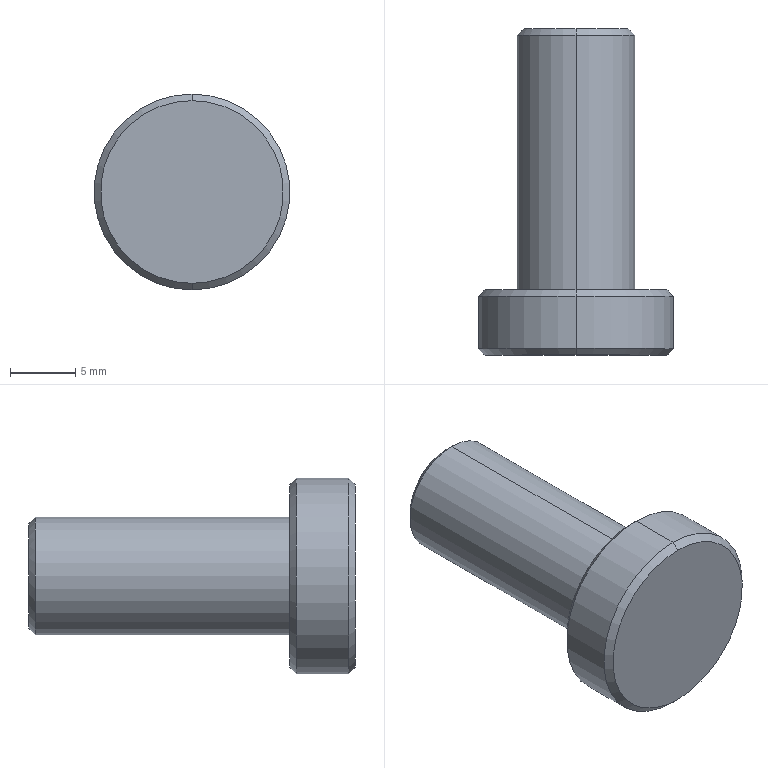Part | SolidWorks | features Chamfer 1, Revolution 1 | 1 solid | 13 faces | box 15 x 25 x 15 mm | volume 2141 mm3 | cone 6 | cylinder 4 | plane 3 | commonest cylinder face diameters 9 x2 15 x2
STEP:
#1=CARTESIAN_POINT('',(0.,25.,4.));
#2=VERTEX_POINT('',#1);
#3=CARTESIAN_POINT('',(0.,25.,-4.));
#4=VERTEX_POINT('',#3);
#5=CARTESIAN_POINT('',(0.,25.,0.));
#6=DIRECTION('',(0.,1.,0.));
#7=DIRECTION('',(0.,0.,1.));
#8=AXIS2_PLACEMENT_3D('',#5,#6,#7);
#9=CIRCLE('',#8,4.);
#10=EDGE_CURVE('',#2,#4,#9,.T.);
#11=ORIENTED_EDGE('',*,*,#10,.F.);
#12=CARTESIAN_POINT('',(0.,24.5,4.5));
#13=VERTEX_POINT('',#12);
#14=CARTESIAN_POINT('',(0.,24.5,4.5));
#15=DIRECTION('',(0.,-0.7071,0.7071));
#16=VECTOR('',#15,1000.);
#17=LINE('',#14,#16);
#18=EDGE_CURVE('',#2,#13,#17,.T.);
#19=ORIENTED_EDGE('',*,*,#18,.T.);
#20=CARTESIAN_POINT('',(0.,24.5,-4.5));
#21=VERTEX_POINT('',#20);
#22=CARTESIAN_POINT('',(0.,24.5,0.));
#23=DIRECTION('',(0.,-1.,0.));
#24=DIRECTION('',(0.,0.,1.));
#25=AXIS2_PLACEMENT_3D('',#22,#23,#24);
#26=CIRCLE('',#25,4.5);
#27=EDGE_CURVE('',#21,#13,#26,.T.);
#28=ORIENTED_EDGE('',*,*,#27,.F.);
#29=CARTESIAN_POINT('',(0.,24.5,-4.5));
#30=DIRECTION('',(0.,-0.7071,-0.7071));
#31=VECTOR('',#30,1000.);
#32=LINE('',#29,#31);
#33=EDGE_CURVE('',#4,#21,#32,.T.);
#34=ORIENTED_EDGE('',*,*,#33,.F.);
#35=EDGE_LOOP('',(#11,#19,#28,#34));
#36=FACE_OUTER_BOUND('',#35,.T.);
#37=CARTESIAN_POINT('',(0.,24.5,0.));
#38=DIRECTION('',(0.,-1.,0.));
#39=DIRECTION('',(0.,0.,-1.));
#40=AXIS2_PLACEMENT_3D('',#37,#38,#39);
#41=CONICAL_SURFACE('',#40,4.5,0.7854);
#42=ADVANCED_FACE('',(#36),#41,.T.);
#43=CARTESIAN_POINT('',(0.,5.,7.));
#44=VERTEX_POINT('',#43);
#45=CARTESIAN_POINT('',(0.,5.,-7.));
#46=VERTEX_POINT('',#45);
#47=CARTESIAN_POINT('',(0.,5.,0.));
#48=DIRECTION('',(0.,1.,0.));
#49=DIRECTION('',(0.,0.,1.));
#50=AXIS2_PLACEMENT_3D('',#47,#48,#49);
#51=CIRCLE('',#50,7.);
#52=EDGE_CURVE('',#44,#46,#51,.T.);
#53=ORIENTED_EDGE('',*,*,#52,.F.);
#54=CARTESIAN_POINT('',(0.,4.5,7.5));
#55=VERTEX_POINT('',#54);
#56=CARTESIAN_POINT('',(0.,4.5,7.5));
#57=DIRECTION('',(0.,-0.7071,0.7071));
#58=VECTOR('',#57,1000.);
#59=LINE('',#56,#58);
#60=EDGE_CURVE('',#44,#55,#59,.T.);
#61=ORIENTED_EDGE('',*,*,#60,.T.);
#62=CARTESIAN_POINT('',(0.,4.5,-7.5));
#63=VERTEX_POINT('',#62);
#64=CARTESIAN_POINT('',(0.,4.5,0.));
#65=DIRECTION('',(0.,-1.,0.));
#66=DIRECTION('',(0.,0.,1.));
#67=AXIS2_PLACEMENT_3D('',#64,#65,#66);
#68=CIRCLE('',#67,7.5);
#69=EDGE_CURVE('',#63,#55,#68,.T.);
#70=ORIENTED_EDGE('',*,*,#69,.F.);
#71=CARTESIAN_POINT('',(0.,4.5,-7.5));
#72=DIRECTION('',(0.,-0.7071,-0.7071));
#73=VECTOR('',#72,1000.);
#74=LINE('',#71,#73);
#75=EDGE_CURVE('',#46,#63,#74,.T.);
#76=ORIENTED_EDGE('',*,*,#75,.F.);
#77=EDGE_LOOP('',(#53,#61,#70,#76));
#78=FACE_OUTER_BOUND('',#77,.T.);
#79=CARTESIAN_POINT('',(0.,4.5,0.));
#80=DIRECTION('',(0.,-1.,0.));
#81=DIRECTION('',(0.,0.,-1.));
#82=AXIS2_PLACEMENT_3D('',#79,#80,#81);
#83=CONICAL_SURFACE('',#82,7.5,0.7854);
#84=ADVANCED_FACE('',(#78),#83,.T.);
#85=CARTESIAN_POINT('',(0.,0.,-7.));
#86=VERTEX_POINT('',#85);
#87=CARTESIAN_POINT('',(0.,0.,7.));
#88=VERTEX_POINT('',#87);
#89=CARTESIAN_POINT('',(0.,0.,0.));
#90=DIRECTION('',(0.,-1.,0.));
#91=DIRECTION('',(0.,0.,-1.));
#92=AXIS2_PLACEMENT_3D('',#89,#90,#91);
#93=CIRCLE('',#92,7.);
#94=EDGE_CURVE('',#86,#88,#93,.T.);
#95=ORIENTED_EDGE('',*,*,#94,.F.);
#96=CARTESIAN_POINT('',(0.,0.5,-7.5));
#97=VERTEX_POINT('',#96);
#98=CARTESIAN_POINT('',(0.,0.,-7.));
#99=DIRECTION('',(0.,0.7071,-0.7071));
#100=VECTOR('',#99,1000.);
#101=LINE('',#98,#100);
#102=EDGE_CURVE('',#86,#97,#101,.T.);
#103=ORIENTED_EDGE('',*,*,#102,.T.);
#104=CARTESIAN_POINT('',(0.,0.5,7.5));
#105=VERTEX_POINT('',#104);
#106=CARTESIAN_POINT('',(0.,0.5,0.));
#107=DIRECTION('',(0.,1.,0.));
#108=DIRECTION('',(0.,0.,-1.));
#109=AXIS2_PLACEMENT_3D('',#106,#107,#108);
#110=CIRCLE('',#109,7.5);
#111=EDGE_CURVE('',#105,#97,#110,.T.);
#112=ORIENTED_EDGE('',*,*,#111,.F.);
#113=CARTESIAN_POINT('',(0.,0.,7.));
#114=DIRECTION('',(0.,0.7071,0.7071));
#115=VECTOR('',#114,1000.);
#116=LINE('',#113,#115);
#117=EDGE_CURVE('',#88,#105,#116,.T.);
#118=ORIENTED_EDGE('',*,*,#117,.F.);
#119=EDGE_LOOP('',(#95,#103,#112,#118));
#120=FACE_OUTER_BOUND('',#119,.T.);
#121=CARTESIAN_POINT('',(0.,0.,0.));
#122=DIRECTION('',(0.,1.,0.));
#123=DIRECTION('',(0.,0.,1.));
#124=AXIS2_PLACEMENT_3D('',#121,#122,#123);
#125=CONICAL_SURFACE('',#124,7.,0.7854);
#126=ADVANCED_FACE('',(#120),#125,.T.);
#127=ORIENTED_EDGE('',*,*,#69,.T.);
#128=CARTESIAN_POINT('',(0.,0.,7.5));
#129=DIRECTION('',(0.,-1.,0.));
#130=VECTOR('',#129,1000.);
#131=LINE('',#128,#130);
#132=EDGE_CURVE('',#55,#105,#131,.T.);
#133=ORIENTED_EDGE('',*,*,#132,.T.);
#134=ORIENTED_EDGE('',*,*,#111,.T.);
#135=CARTESIAN_POINT('',(0.,0.,-7.5));
#136=DIRECTION('',(0.,-1.,0.));
#137=VECTOR('',#136,1000.);
#138=LINE('',#135,#137);
#139=EDGE_CURVE('',#63,#97,#138,.T.);
#140=ORIENTED_EDGE('',*,*,#139,.F.);
#141=EDGE_LOOP('',(#127,#133,#134,#140));
#142=FACE_OUTER_BOUND('',#141,.T.);
#143=CARTESIAN_POINT('',(0.,0.,0.));
#144=DIRECTION('',(0.,-1.,0.));
#145=DIRECTION('',(0.,0.,-1.));
#146=AXIS2_PLACEMENT_3D('',#143,#144,#145);
#147=CYLINDRICAL_SURFACE('',#146,7.5);
#148=ADVANCED_FACE('',(#142),#147,.T.);
#149=ORIENTED_EDGE('',*,*,#27,.T.);
#150=CARTESIAN_POINT('',(0.,5.,4.5));
#151=VERTEX_POINT('',#150);
#152=CARTESIAN_POINT('',(0.,0.,4.5));
#153=DIRECTION('',(0.,-1.,0.));
#154=VECTOR('',#153,1000.);
#155=LINE('',#152,#154);
#156=EDGE_CURVE('',#13,#151,#155,.T.);
#157=ORIENTED_EDGE('',*,*,#156,.T.);
#158=CARTESIAN_POINT('',(0.,5.,-4.5));
#159=VERTEX_POINT('',#158);
#160=CARTESIAN_POINT('',(0.,5.,0.));
#161=DIRECTION('',(0.,-1.,0.));
#162=DIRECTION('',(0.,0.,-1.));
#163=AXIS2_PLACEMENT_3D('',#160,#161,#162);
#164=CIRCLE('',#163,4.5);
#165=EDGE_CURVE('',#159,#151,#164,.T.);
#166=ORIENTED_EDGE('',*,*,#165,.F.);
#167=CARTESIAN_POINT('',(0.,0.,-4.5));
#168=DIRECTION('',(0.,-1.,0.));
#169=VECTOR('',#168,1000.);
#170=LINE('',#167,#169);
#171=EDGE_CURVE('',#21,#159,#170,.T.);
#172=ORIENTED_EDGE('',*,*,#171,.F.);
#173=EDGE_LOOP('',(#149,#157,#166,#172));
#174=FACE_OUTER_BOUND('',#173,.T.);
#175=CARTESIAN_POINT('',(0.,0.,0.));
#176=DIRECTION('',(0.,-1.,0.));
#177=DIRECTION('',(0.,0.,-1.));
#178=AXIS2_PLACEMENT_3D('',#175,#176,#177);
#179=CYLINDRICAL_SURFACE('',#178,4.5);
#180=ADVANCED_FACE('',(#174),#179,.T.);
#181=CARTESIAN_POINT('',(0.,25.,0.));
#182=DIRECTION('',(0.,1.,0.));
#183=DIRECTION('',(0.,0.,1.));
#184=AXIS2_PLACEMENT_3D('',#181,#182,#183);
#185=CIRCLE('',#184,4.);
#186=EDGE_CURVE('',#4,#2,#185,.T.);
#187=ORIENTED_EDGE('',*,*,#186,.T.);
#188=ORIENTED_EDGE('',*,*,#10,.T.);
#189=EDGE_LOOP('',(#187,#188));
#190=FACE_OUTER_BOUND('',#189,.T.);
#191=CARTESIAN_POINT('',(0.,25.,0.));
#192=DIRECTION('',(0.,1.,0.));
#193=DIRECTION('',(0.,0.,1.));
#194=AXIS2_PLACEMENT_3D('',#191,#192,#193);
#195=PLANE('',#194);
#196=ADVANCED_FACE('',(#190),#195,.T.);
#197=ORIENTED_EDGE('',*,*,#156,.F.);
#198=CARTESIAN_POINT('',(0.,24.5,0.));
#199=DIRECTION('',(0.,-1.,0.));
#200=DIRECTION('',(0.,0.,1.));
#201=AXIS2_PLACEMENT_3D('',#198,#199,#200);
#202=CIRCLE('',#201,4.5);
#203=EDGE_CURVE('',#13,#21,#202,.T.);
#204=ORIENTED_EDGE('',*,*,#203,.T.);
#205=ORIENTED_EDGE('',*,*,#171,.T.);
#206=CARTESIAN_POINT('',(0.,5.,0.));
#207=DIRECTION('',(0.,-1.,0.));
#208=DIRECTION('',(0.,0.,-1.));
#209=AXIS2_PLACEMENT_3D('',#206,#207,#208);
#210=CIRCLE('',#209,4.5);
#211=EDGE_CURVE('',#151,#159,#210,.T.);
#212=ORIENTED_EDGE('',*,*,#211,.F.);
#213=EDGE_LOOP('',(#197,#204,#205,#212));
#214=FACE_OUTER_BOUND('',#213,.T.);
#215=CARTESIAN_POINT('',(0.,0.,0.));
#216=DIRECTION('',(0.,-1.,0.));
#217=DIRECTION('',(0.,0.,-1.));
#218=AXIS2_PLACEMENT_3D('',#215,#216,#217);
#219=CYLINDRICAL_SURFACE('',#218,4.5);
#220=ADVANCED_FACE('',(#214),#219,.T.);
#221=CARTESIAN_POINT('',(0.,5.,0.));
#222=DIRECTION('',(0.,1.,0.));
#223=DIRECTION('',(0.,0.,1.));
#224=AXIS2_PLACEMENT_3D('',#221,#222,#223);
#225=CIRCLE('',#224,7.);
#226=EDGE_CURVE('',#46,#44,#225,.T.);
#227=ORIENTED_EDGE('',*,*,#226,.T.);
#228=ORIENTED_EDGE('',*,*,#52,.T.);
#229=EDGE_LOOP('',(#227,#228));
#230=FACE_OUTER_BOUND('',#229,.T.);
#231=ORIENTED_EDGE('',*,*,#165,.T.);
#232=ORIENTED_EDGE('',*,*,#211,.T.);
#233=EDGE_LOOP('',(#231,#232));
#234=FACE_BOUND('',#233,.T.);
#235=CARTESIAN_POINT('',(0.,5.,-4.5));
#236=DIRECTION('',(0.,1.,0.));
#237=DIRECTION('',(0.,0.,1.));
#238=AXIS2_PLACEMENT_3D('',#235,#236,#237);
#239=PLANE('',#238);
#240=ADVANCED_FACE('',(#230,#234),#239,.T.);
#241=ORIENTED_EDGE('',*,*,#132,.F.);
#242=CARTESIAN_POINT('',(0.,4.5,0.));
#243=DIRECTION('',(0.,-1.,0.));
#244=DIRECTION('',(0.,0.,1.));
#245=AXIS2_PLACEMENT_3D('',#242,#243,#244);
#246=CIRCLE('',#245,7.5);
#247=EDGE_CURVE('',#55,#63,#246,.T.);
#248=ORIENTED_EDGE('',*,*,#247,.T.);
#249=ORIENTED_EDGE('',*,*,#139,.T.);
#250=CARTESIAN_POINT('',(0.,0.5,0.));
#251=DIRECTION('',(0.,1.,0.));
#252=DIRECTION('',(0.,0.,-1.));
#253=AXIS2_PLACEMENT_3D('',#250,#251,#252);
#254=CIRCLE('',#253,7.5);
#255=EDGE_CURVE('',#97,#105,#254,.T.);
#256=ORIENTED_EDGE('',*,*,#255,.T.);
#257=EDGE_LOOP('',(#241,#248,#249,#256));
#258=FACE_OUTER_BOUND('',#257,.T.);
#259=CARTESIAN_POINT('',(0.,0.,0.));
#260=DIRECTION('',(0.,-1.,0.));
#261=DIRECTION('',(0.,0.,-1.));
#262=AXIS2_PLACEMENT_3D('',#259,#260,#261);
#263=CYLINDRICAL_SURFACE('',#262,7.5);
#264=ADVANCED_FACE('',(#258),#263,.T.);
#265=CARTESIAN_POINT('',(0.,0.,0.));
#266=DIRECTION('',(0.,-1.,0.));
#267=DIRECTION('',(0.,0.,-1.));
#268=AXIS2_PLACEMENT_3D('',#265,#266,#267);
#269=CIRCLE('',#268,7.);
#270=EDGE_CURVE('',#88,#86,#269,.T.);
#271=ORIENTED_EDGE('',*,*,#270,.T.);
#272=ORIENTED_EDGE('',*,*,#94,.T.);
#273=EDGE_LOOP('',(#271,#272));
#274=FACE_OUTER_BOUND('',#273,.T.);
#275=CARTESIAN_POINT('',(0.,0.,-7.5));
#276=DIRECTION('',(0.,-1.,0.));
#277=DIRECTION('',(0.,0.,-1.));
#278=AXIS2_PLACEMENT_3D('',#275,#276,#277);
#279=PLANE('',#278);
#280=ADVANCED_FACE('',(#274),#279,.T.);
#281=ORIENTED_EDGE('',*,*,#102,.F.);
#282=ORIENTED_EDGE('',*,*,#270,.F.);
#283=ORIENTED_EDGE('',*,*,#117,.T.);
#284=ORIENTED_EDGE('',*,*,#255,.F.);
#285=EDGE_LOOP('',(#281,#282,#283,#284));
#286=FACE_OUTER_BOUND('',#285,.T.);
#287=CARTESIAN_POINT('',(0.,0.,0.));
#288=DIRECTION('',(0.,1.,0.));
#289=DIRECTION('',(0.,0.,1.));
#290=AXIS2_PLACEMENT_3D('',#287,#288,#289);
#291=CONICAL_SURFACE('',#290,7.,0.7854);
#292=ADVANCED_FACE('',(#286),#291,.T.);
#293=ORIENTED_EDGE('',*,*,#60,.F.);
#294=ORIENTED_EDGE('',*,*,#226,.F.);
#295=ORIENTED_EDGE('',*,*,#75,.T.);
#296=ORIENTED_EDGE('',*,*,#247,.F.);
#297=EDGE_LOOP('',(#293,#294,#295,#296));
#298=FACE_OUTER_BOUND('',#297,.T.);
#299=CARTESIAN_POINT('',(0.,4.5,0.));
#300=DIRECTION('',(0.,-1.,0.));
#301=DIRECTION('',(0.,0.,-1.));
#302=AXIS2_PLACEMENT_3D('',#299,#300,#301);
#303=CONICAL_SURFACE('',#302,7.5,0.7854);
#304=ADVANCED_FACE('',(#298),#303,.T.);
#305=ORIENTED_EDGE('',*,*,#18,.F.);
#306=ORIENTED_EDGE('',*,*,#186,.F.);
#307=ORIENTED_EDGE('',*,*,#33,.T.);
#308=ORIENTED_EDGE('',*,*,#203,.F.);
#309=EDGE_LOOP('',(#305,#306,#307,#308));
#310=FACE_OUTER_BOUND('',#309,.T.);
#311=CARTESIAN_POINT('',(0.,24.5,0.));
#312=DIRECTION('',(0.,-1.,0.));
#313=DIRECTION('',(0.,0.,-1.));
#314=AXIS2_PLACEMENT_3D('',#311,#312,#313);
#315=CONICAL_SURFACE('',#314,4.5,0.7854);
#316=ADVANCED_FACE('',(#310),#315,.T.);
#317=CLOSED_SHELL('',(#42,#84,#126,#148,#180,#196,#220,#240,#264,#280,#292,#304,#316));
#318=MANIFOLD_SOLID_BREP('',#317);
#319=CARTESIAN_POINT('',(0.,0.,0.));
#320=DIRECTION('',(0.,0.,1.));
#321=DIRECTION('',(1.,0.,0.));
#322=AXIS2_PLACEMENT_3D('',#319,#320,#321);
#323=(LENGTH_UNIT()NAMED_UNIT(*)SI_UNIT(.MILLI.,.METRE.));
#324=UNCERTAINTY_MEASURE_WITH_UNIT(LENGTH_MEASURE(0.00001),#323,'','');
#325=(NAMED_UNIT(*)PLANE_ANGLE_UNIT()SI_UNIT($,.RADIAN.));
#326=(NAMED_UNIT(*)SI_UNIT($,.STERADIAN.)SOLID_ANGLE_UNIT());
#327=(GEOMETRIC_REPRESENTATION_CONTEXT(3)GLOBAL_UNCERTAINTY_ASSIGNED_CONTEXT((#324))GLOBAL_UNIT_ASSIGNED_CONTEXT((#323,#325,#326))REPRESENTATION_CONTEXT('',''));
#328=ADVANCED_BREP_SHAPE_REPRESENTATION('',(#318,#322),#327);